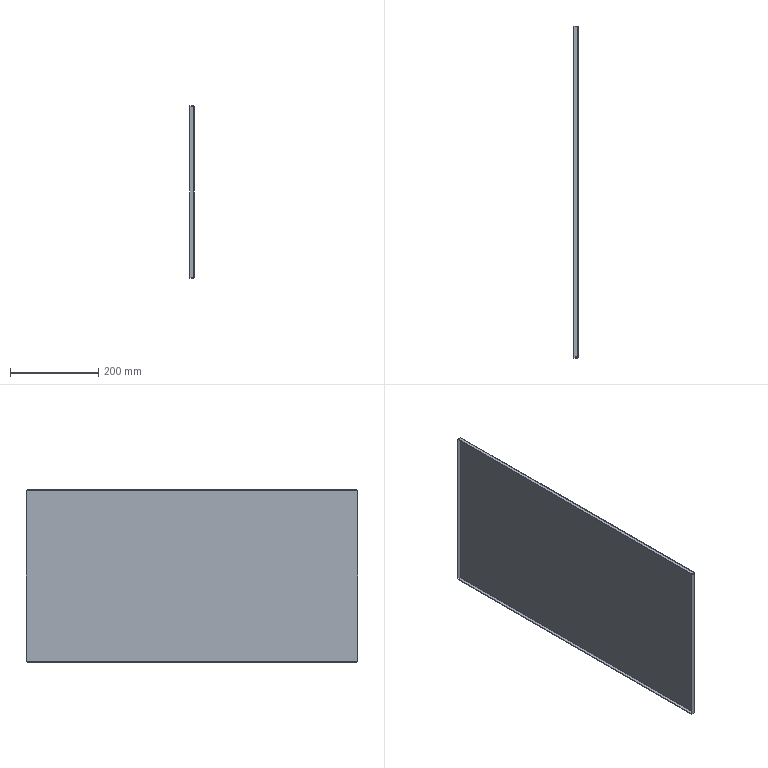Part | SolidWorks | 1 solid | 38 faces | box 10 x 752.001 x 390.001 mm | volume 467554 mm3 | plane 22 | spline 8 | cylinder 8 | commonest cylinder face diameters 0.2 x4 3.2 x4
STEP:
#1=CARTESIAN_POINT('',(-1.5,-374.4,-193.4));
#2=VERTEX_POINT('',#1);
#3=CARTESIAN_POINT('',(-1.5,374.4,-193.4));
#4=VERTEX_POINT('',#3);
#5=CARTESIAN_POINT('',(-1.5,-374.4,-193.4));
#6=DIRECTION('',(0.,1.,0.));
#7=VECTOR('',#6,1000.);
#8=LINE('',#5,#7);
#9=EDGE_CURVE('',#2,#4,#8,.T.);
#10=ORIENTED_EDGE('',*,*,#9,.F.);
#11=CARTESIAN_POINT('',(-1.5,-374.4,193.4));
#12=VERTEX_POINT('',#11);
#13=CARTESIAN_POINT('',(-1.5,-374.4,193.4));
#14=DIRECTION('',(0.,0.,-1.));
#15=VECTOR('',#14,1000.);
#16=LINE('',#13,#15);
#17=EDGE_CURVE('',#12,#2,#16,.T.);
#18=ORIENTED_EDGE('',*,*,#17,.F.);
#19=CARTESIAN_POINT('',(-1.5,374.4,193.4));
#20=VERTEX_POINT('',#19);
#21=CARTESIAN_POINT('',(-1.5,374.4,193.4));
#22=DIRECTION('',(0.,-1.,0.));
#23=VECTOR('',#22,1000.);
#24=LINE('',#21,#23);
#25=EDGE_CURVE('',#20,#12,#24,.T.);
#26=ORIENTED_EDGE('',*,*,#25,.F.);
#27=CARTESIAN_POINT('',(-1.5,374.4,-193.4));
#28=DIRECTION('',(0.,0.,1.));
#29=VECTOR('',#28,1000.);
#30=LINE('',#27,#29);
#31=EDGE_CURVE('',#4,#20,#30,.T.);
#32=ORIENTED_EDGE('',*,*,#31,.F.);
#33=EDGE_LOOP('',(#10,#18,#26,#32));
#34=FACE_OUTER_BOUND('',#33,.T.);
#35=CARTESIAN_POINT('',(-1.5,0.,0.));
#36=DIRECTION('',(1.,0.,0.));
#37=DIRECTION('',(0.,0.,-1.));
#38=AXIS2_PLACEMENT_3D('',#35,#36,#37);
#39=PLANE('',#38);
#40=ADVANCED_FACE('',(#34),#39,.F.);
#41=CARTESIAN_POINT('',(0.,-374.4,193.4));
#42=VERTEX_POINT('',#41);
#43=CARTESIAN_POINT('',(0.,-374.4,-193.4));
#44=VERTEX_POINT('',#43);
#45=CARTESIAN_POINT('',(0.,-374.4,193.4));
#46=DIRECTION('',(0.,0.,-1.));
#47=VECTOR('',#46,1000.);
#48=LINE('',#45,#47);
#49=EDGE_CURVE('',#42,#44,#48,.T.);
#50=ORIENTED_EDGE('',*,*,#49,.T.);
#51=CARTESIAN_POINT('',(0.,374.4,-193.4));
#52=VERTEX_POINT('',#51);
#53=CARTESIAN_POINT('',(0.,-374.4,-193.4));
#54=DIRECTION('',(0.,1.,0.));
#55=VECTOR('',#54,1000.);
#56=LINE('',#53,#55);
#57=EDGE_CURVE('',#44,#52,#56,.T.);
#58=ORIENTED_EDGE('',*,*,#57,.T.);
#59=CARTESIAN_POINT('',(0.,374.4,193.4));
#60=VERTEX_POINT('',#59);
#61=CARTESIAN_POINT('',(0.,374.4,-193.4));
#62=DIRECTION('',(0.,0.,1.));
#63=VECTOR('',#62,1000.);
#64=LINE('',#61,#63);
#65=EDGE_CURVE('',#52,#60,#64,.T.);
#66=ORIENTED_EDGE('',*,*,#65,.T.);
#67=CARTESIAN_POINT('',(0.,374.4,193.4));
#68=DIRECTION('',(0.,-1.,0.));
#69=VECTOR('',#68,1000.);
#70=LINE('',#67,#69);
#71=EDGE_CURVE('',#60,#42,#70,.T.);
#72=ORIENTED_EDGE('',*,*,#71,.T.);
#73=EDGE_LOOP('',(#50,#58,#66,#72));
#74=FACE_OUTER_BOUND('',#73,.T.);
#75=CARTESIAN_POINT('',(0.,0.,0.));
#76=DIRECTION('',(1.,0.,0.));
#77=DIRECTION('',(0.,0.,-1.));
#78=AXIS2_PLACEMENT_3D('',#75,#76,#77);
#79=PLANE('',#78);
#80=ADVANCED_FACE('',(#74),#79,.T.);
#81=CARTESIAN_POINT('',(-1.6,376.,192.793));
#82=VERTEX_POINT('',#81);
#83=CARTESIAN_POINT('',(-1.6,374.5,192.793));
#84=VERTEX_POINT('',#83);
#85=CARTESIAN_POINT('',(-1.6,374.5,192.793));
#86=DIRECTION('',(0.,-1.,0.));
#87=VECTOR('',#86,1000.);
#88=LINE('',#85,#87);
#89=EDGE_CURVE('',#82,#84,#88,.T.);
#90=ORIENTED_EDGE('',*,*,#89,.T.);
#91=CARTESIAN_POINT('',(-1.5,374.4,193.4));
#92=CARTESIAN_POINT('',(-1.5,374.426,193.299));
#93=CARTESIAN_POINT('',(-1.511,374.452,193.198));
#94=CARTESIAN_POINT('',(-1.548,374.489,192.995));
#95=CARTESIAN_POINT('',(-1.574,374.5,192.894));
#96=CARTESIAN_POINT('',(-1.6,374.5,192.793));
#97=B_SPLINE_CURVE_WITH_KNOTS('',3,(#91,#92,#93,#94,#95,#96),.UNSPECIFIED.,.F.,.F.,(4,2,4),(0.,0.5,1.),.UNSPECIFIED.);
#98=EDGE_CURVE('',#20,#84,#97,.T.);
#99=ORIENTED_EDGE('',*,*,#98,.F.);
#100=CARTESIAN_POINT('',(-1.5,374.4,193.4));
#101=DIRECTION('',(1.,0.,0.));
#102=VECTOR('',#101,1000.);
#103=LINE('',#100,#102);
#104=EDGE_CURVE('',#20,#60,#103,.T.);
#105=ORIENTED_EDGE('',*,*,#104,.T.);
#106=CARTESIAN_POINT('',(0.,374.4,193.4));
#107=CARTESIAN_POINT('',(0.,374.612,193.349));
#108=CARTESIAN_POINT('',(-0.04048,374.815,193.3));
#109=CARTESIAN_POINT('',(-0.2012,375.205,193.198));
#110=CARTESIAN_POINT('',(-0.3186,375.381,193.148));
#111=CARTESIAN_POINT('',(-0.5418,375.605,193.071));
#112=CARTESIAN_POINT('',(-0.6225,375.671,193.046));
#113=CARTESIAN_POINT('',(-0.7959,375.787,192.996));
#114=CARTESIAN_POINT('',(-0.8897,375.838,192.97));
#115=CARTESIAN_POINT('',(-1.18,375.958,192.894));
#116=CARTESIAN_POINT('',(-1.388,376.,192.844));
#117=CARTESIAN_POINT('',(-1.6,376.,192.793));
#118=B_SPLINE_CURVE_WITH_KNOTS('',3,(#106,#107,#108,#109,#110,#111,#112,#113,#114,#115,#116,#117),.UNSPECIFIED.,.F.,.F.,(4,2,2,2,2,4),(0.,0.0006399,0.00128,0.0016,0.00192,0.00256),.UNSPECIFIED.);
#119=EDGE_CURVE('',#60,#82,#118,.T.);
#120=ORIENTED_EDGE('',*,*,#119,.T.);
#121=EDGE_LOOP('',(#90,#99,#105,#120));
#122=FACE_OUTER_BOUND('',#121,.T.);
#123=CARTESIAN_POINT('',(0.015,374.4,193.4));
#124=CARTESIAN_POINT('',(0.015,374.611,193.349));
#125=CARTESIAN_POINT('',(-0.02703,374.823,193.299));
#126=CARTESIAN_POINT('',(-0.1888,375.213,193.198));
#127=CARTESIAN_POINT('',(-0.3085,375.392,193.147));
#128=CARTESIAN_POINT('',(-0.6075,375.691,193.046));
#129=CARTESIAN_POINT('',(-0.7867,375.811,192.995));
#130=CARTESIAN_POINT('',(-1.177,375.973,192.894));
#131=CARTESIAN_POINT('',(-1.389,376.015,192.843));
#132=CARTESIAN_POINT('',(-1.6,376.015,192.793));
#133=CARTESIAN_POINT('',(0.,374.4,193.4));
#134=CARTESIAN_POINT('',(0.,374.609,193.349));
#135=CARTESIAN_POINT('',(-0.04164,374.819,193.299));
#136=CARTESIAN_POINT('',(-0.2019,375.206,193.198));
#137=CARTESIAN_POINT('',(-0.3205,375.383,193.147));
#138=CARTESIAN_POINT('',(-0.6167,375.679,193.046));
#139=CARTESIAN_POINT('',(-0.7942,375.798,192.995));
#140=CARTESIAN_POINT('',(-1.181,375.958,192.894));
#141=CARTESIAN_POINT('',(-1.391,376.,192.843));
#142=CARTESIAN_POINT('',(-1.6,376.,192.793));
#143=CARTESIAN_POINT('',(-1.5,374.4,193.4));
#144=CARTESIAN_POINT('',(-1.5,374.413,193.349));
#145=CARTESIAN_POINT('',(-1.503,374.426,193.299));
#146=CARTESIAN_POINT('',(-1.513,374.45,193.198));
#147=CARTESIAN_POINT('',(-1.52,374.461,193.147));
#148=CARTESIAN_POINT('',(-1.539,374.48,193.046));
#149=CARTESIAN_POINT('',(-1.55,374.487,192.995));
#150=CARTESIAN_POINT('',(-1.574,374.497,192.894));
#151=CARTESIAN_POINT('',(-1.587,374.5,192.843));
#152=CARTESIAN_POINT('',(-1.6,374.5,192.793));
#153=B_SPLINE_SURFACE_WITH_KNOTS('',1,3,((#123,#124,#125,#126,#127,#128,#129,#130,#131,#132),(#133,#134,#135,#136,#137,#138,#139,#140,#141,#142),(#143,#144,#145,#146,#147,#148,#149,#150,#151,#152)),.UNSPECIFIED.,.F.,.F.,.F.,(2,1,2),(4,2,2,2,4),(-0.01,0.,1.),(0.,0.25,0.5,0.75,1.),.UNSPECIFIED.);
#154=ADVANCED_FACE('',(#122),#153,.F.);
#155=CARTESIAN_POINT('',(-1.6,374.5,-192.793));
#156=VERTEX_POINT('',#155);
#157=CARTESIAN_POINT('',(-1.6,374.5,-192.793));
#158=CARTESIAN_POINT('',(-1.574,374.5,-192.894));
#159=CARTESIAN_POINT('',(-1.548,374.489,-192.995));
#160=CARTESIAN_POINT('',(-1.511,374.452,-193.198));
#161=CARTESIAN_POINT('',(-1.5,374.426,-193.299));
#162=CARTESIAN_POINT('',(-1.5,374.4,-193.4));
#163=B_SPLINE_CURVE_WITH_KNOTS('',3,(#157,#158,#159,#160,#161,#162),.UNSPECIFIED.,.F.,.F.,(4,2,4),(0.,0.5,1.),.UNSPECIFIED.);
#164=EDGE_CURVE('',#156,#4,#163,.T.);
#165=ORIENTED_EDGE('',*,*,#164,.F.);
#166=CARTESIAN_POINT('',(-1.6,376.,-192.793));
#167=VERTEX_POINT('',#166);
#168=CARTESIAN_POINT('',(-1.6,374.5,-192.793));
#169=DIRECTION('',(0.,-1.,0.));
#170=VECTOR('',#169,1000.);
#171=LINE('',#168,#170);
#172=EDGE_CURVE('',#167,#156,#171,.T.);
#173=ORIENTED_EDGE('',*,*,#172,.F.);
#174=CARTESIAN_POINT('',(-1.6,376.,-192.793));
#175=CARTESIAN_POINT('',(-1.388,376.,-192.844));
#176=CARTESIAN_POINT('',(-1.185,375.96,-192.893));
#177=CARTESIAN_POINT('',(-0.7952,375.799,-192.995));
#178=CARTESIAN_POINT('',(-0.619,375.681,-193.045));
#179=CARTESIAN_POINT('',(-0.3953,375.458,-193.121));
#180=CARTESIAN_POINT('',(-0.329,375.378,-193.147));
#181=CARTESIAN_POINT('',(-0.2128,375.204,-193.197));
#182=CARTESIAN_POINT('',(-0.1625,375.11,-193.223));
#183=CARTESIAN_POINT('',(-0.04195,374.82,-193.299));
#184=CARTESIAN_POINT('',(0.,374.612,-193.349));
#185=CARTESIAN_POINT('',(0.,374.4,-193.4));
#186=B_SPLINE_CURVE_WITH_KNOTS('',3,(#174,#175,#176,#177,#178,#179,#180,#181,#182,#183,#184,#185),.UNSPECIFIED.,.F.,.F.,(4,2,2,2,2,4),(0.,0.0006399,0.00128,0.0016,0.00192,0.00256),.UNSPECIFIED.);
#187=EDGE_CURVE('',#167,#52,#186,.T.);
#188=ORIENTED_EDGE('',*,*,#187,.T.);
#189=CARTESIAN_POINT('',(-1.5,374.4,-193.4));
#190=DIRECTION('',(1.,0.,0.));
#191=VECTOR('',#190,1000.);
#192=LINE('',#189,#191);
#193=EDGE_CURVE('',#4,#52,#192,.T.);
#194=ORIENTED_EDGE('',*,*,#193,.F.);
#195=EDGE_LOOP('',(#165,#173,#188,#194));
#196=FACE_OUTER_BOUND('',#195,.T.);
#197=CARTESIAN_POINT('',(-1.6,376.015,-192.793));
#198=CARTESIAN_POINT('',(-1.389,376.015,-192.843));
#199=CARTESIAN_POINT('',(-1.177,375.973,-192.894));
#200=CARTESIAN_POINT('',(-0.7867,375.811,-192.995));
#201=CARTESIAN_POINT('',(-0.6075,375.691,-193.046));
#202=CARTESIAN_POINT('',(-0.3085,375.392,-193.147));
#203=CARTESIAN_POINT('',(-0.1888,375.213,-193.198));
#204=CARTESIAN_POINT('',(-0.02703,374.823,-193.299));
#205=CARTESIAN_POINT('',(0.015,374.611,-193.349));
#206=CARTESIAN_POINT('',(0.015,374.4,-193.4));
#207=CARTESIAN_POINT('',(-1.6,376.,-192.793));
#208=CARTESIAN_POINT('',(-1.391,376.,-192.843));
#209=CARTESIAN_POINT('',(-1.181,375.958,-192.894));
#210=CARTESIAN_POINT('',(-0.7942,375.798,-192.995));
#211=CARTESIAN_POINT('',(-0.6167,375.679,-193.046));
#212=CARTESIAN_POINT('',(-0.3205,375.383,-193.147));
#213=CARTESIAN_POINT('',(-0.2019,375.206,-193.198));
#214=CARTESIAN_POINT('',(-0.04164,374.819,-193.299));
#215=CARTESIAN_POINT('',(0.,374.609,-193.349));
#216=CARTESIAN_POINT('',(0.,374.4,-193.4));
#217=CARTESIAN_POINT('',(-1.6,374.5,-192.793));
#218=CARTESIAN_POINT('',(-1.587,374.5,-192.843));
#219=CARTESIAN_POINT('',(-1.574,374.497,-192.894));
#220=CARTESIAN_POINT('',(-1.55,374.487,-192.995));
#221=CARTESIAN_POINT('',(-1.539,374.48,-193.046));
#222=CARTESIAN_POINT('',(-1.52,374.461,-193.147));
#223=CARTESIAN_POINT('',(-1.513,374.45,-193.198));
#224=CARTESIAN_POINT('',(-1.503,374.426,-193.299));
#225=CARTESIAN_POINT('',(-1.5,374.413,-193.349));
#226=CARTESIAN_POINT('',(-1.5,374.4,-193.4));
#227=B_SPLINE_SURFACE_WITH_KNOTS('',1,3,((#197,#198,#199,#200,#201,#202,#203,#204,#205,#206),(#207,#208,#209,#210,#211,#212,#213,#214,#215,#216),(#217,#218,#219,#220,#221,#222,#223,#224,#225,#226)),.UNSPECIFIED.,.F.,.F.,.F.,(2,1,2),(4,2,2,2,4),(-0.01,0.,1.),(0.,0.25,0.5,0.75,1.),.UNSPECIFIED.);
#228=ADVANCED_FACE('',(#196),#227,.F.);
#229=ORIENTED_EDGE('',*,*,#65,.F.);
#230=ORIENTED_EDGE('',*,*,#187,.F.);
#231=CARTESIAN_POINT('',(-1.6,376.,0.));
#232=DIRECTION('',(0.,0.,-1.));
#233=VECTOR('',#232,1000.);
#234=LINE('',#231,#233);
#235=EDGE_CURVE('',#82,#167,#234,.T.);
#236=ORIENTED_EDGE('',*,*,#235,.F.);
#237=ORIENTED_EDGE('',*,*,#119,.F.);
#238=EDGE_LOOP('',(#229,#230,#236,#237));
#239=FACE_OUTER_BOUND('',#238,.T.);
#240=CARTESIAN_POINT('',(-1.6,374.4,-193.4));
#241=DIRECTION('',(0.,0.,-1.));
#242=DIRECTION('',(0.,1.,0.));
#243=AXIS2_PLACEMENT_3D('',#240,#241,#242);
#244=CYLINDRICAL_SURFACE('',#243,1.6);
#245=ADVANCED_FACE('',(#239),#244,.T.);
#246=ORIENTED_EDGE('',*,*,#31,.T.);
#247=ORIENTED_EDGE('',*,*,#98,.T.);
#248=CARTESIAN_POINT('',(-1.6,374.5,195.));
#249=DIRECTION('',(0.,0.,-1.));
#250=VECTOR('',#249,1000.);
#251=LINE('',#248,#250);
#252=EDGE_CURVE('',#84,#156,#251,.T.);
#253=ORIENTED_EDGE('',*,*,#252,.T.);
#254=ORIENTED_EDGE('',*,*,#164,.T.);
#255=EDGE_LOOP('',(#246,#247,#253,#254));
#256=FACE_OUTER_BOUND('',#255,.T.);
#257=CARTESIAN_POINT('',(-1.6,374.4,-193.4));
#258=DIRECTION('',(0.,0.,-1.));
#259=DIRECTION('',(0.,1.,0.));
#260=AXIS2_PLACEMENT_3D('',#257,#258,#259);
#261=CYLINDRICAL_SURFACE('',#260,0.1);
#262=ADVANCED_FACE('',(#256),#261,.F.);
#263=CARTESIAN_POINT('',(-10.,374.5,192.793));
#264=VERTEX_POINT('',#263);
#265=CARTESIAN_POINT('',(-10.,376.,192.793));
#266=VERTEX_POINT('',#265);
#267=CARTESIAN_POINT('',(-10.,376.,192.793));
#268=DIRECTION('',(0.,1.,0.));
#269=VECTOR('',#268,1000.);
#270=LINE('',#267,#269);
#271=EDGE_CURVE('',#264,#266,#270,.T.);
#272=ORIENTED_EDGE('',*,*,#271,.F.);
#273=CARTESIAN_POINT('',(0.,374.5,192.793));
#274=DIRECTION('',(-1.,0.,0.));
#275=VECTOR('',#274,1000.);
#276=LINE('',#273,#275);
#277=EDGE_CURVE('',#84,#264,#276,.T.);
#278=ORIENTED_EDGE('',*,*,#277,.F.);
#279=ORIENTED_EDGE('',*,*,#89,.F.);
#280=CARTESIAN_POINT('',(0.,376.,192.793));
#281=DIRECTION('',(1.,0.,0.));
#282=VECTOR('',#281,1000.);
#283=LINE('',#280,#282);
#284=EDGE_CURVE('',#266,#82,#283,.T.);
#285=ORIENTED_EDGE('',*,*,#284,.F.);
#286=EDGE_LOOP('',(#272,#278,#279,#285));
#287=FACE_OUTER_BOUND('',#286,.T.);
#288=CARTESIAN_POINT('',(-1.5,374.5,192.793));
#289=DIRECTION('',(0.,0.,1.));
#290=DIRECTION('',(1.,0.,0.));
#291=AXIS2_PLACEMENT_3D('',#288,#289,#290);
#292=PLANE('',#291);
#293=ADVANCED_FACE('',(#287),#292,.T.);
#294=CARTESIAN_POINT('',(-10.,376.,-192.793));
#295=VERTEX_POINT('',#294);
#296=CARTESIAN_POINT('',(-1.5,376.,-192.793));
#297=DIRECTION('',(1.,0.,0.));
#298=VECTOR('',#297,1000.);
#299=LINE('',#296,#298);
#300=EDGE_CURVE('',#295,#167,#299,.T.);
#301=ORIENTED_EDGE('',*,*,#300,.F.);
#302=CARTESIAN_POINT('',(-10.,376.,-195.));
#303=DIRECTION('',(0.,0.,-1.));
#304=VECTOR('',#303,1000.);
#305=LINE('',#302,#304);
#306=EDGE_CURVE('',#266,#295,#305,.T.);
#307=ORIENTED_EDGE('',*,*,#306,.F.);
#308=ORIENTED_EDGE('',*,*,#284,.T.);
#309=ORIENTED_EDGE('',*,*,#235,.T.);
#310=EDGE_LOOP('',(#301,#307,#308,#309));
#311=FACE_OUTER_BOUND('',#310,.T.);
#312=CARTESIAN_POINT('',(0.,376.,0.));
#313=DIRECTION('',(0.,1.,0.));
#314=DIRECTION('',(-1.,0.,0.));
#315=AXIS2_PLACEMENT_3D('',#312,#313,#314);
#316=PLANE('',#315);
#317=ADVANCED_FACE('',(#311),#316,.T.);
#318=CARTESIAN_POINT('',(-10.,374.5,-192.793));
#319=VERTEX_POINT('',#318);
#320=CARTESIAN_POINT('',(-10.,374.5,0.));
#321=DIRECTION('',(0.,0.,-1.));
#322=VECTOR('',#321,1000.);
#323=LINE('',#320,#322);
#324=EDGE_CURVE('',#264,#319,#323,.T.);
#325=ORIENTED_EDGE('',*,*,#324,.T.);
#326=CARTESIAN_POINT('',(-1.5,374.5,-192.793));
#327=DIRECTION('',(-1.,0.,0.));
#328=VECTOR('',#327,1000.);
#329=LINE('',#326,#328);
#330=EDGE_CURVE('',#156,#319,#329,.T.);
#331=ORIENTED_EDGE('',*,*,#330,.F.);
#332=ORIENTED_EDGE('',*,*,#252,.F.);
#333=ORIENTED_EDGE('',*,*,#277,.T.);
#334=EDGE_LOOP('',(#325,#331,#332,#333));
#335=FACE_OUTER_BOUND('',#334,.T.);
#336=CARTESIAN_POINT('',(0.,374.5,0.));
#337=DIRECTION('',(0.,1.,0.));
#338=DIRECTION('',(-1.,0.,0.));
#339=AXIS2_PLACEMENT_3D('',#336,#337,#338);
#340=PLANE('',#339);
#341=ADVANCED_FACE('',(#335),#340,.F.);
#342=CARTESIAN_POINT('',(-10.,374.5,-192.793));
#343=DIRECTION('',(0.,1.,0.));
#344=VECTOR('',#343,1000.);
#345=LINE('',#342,#344);
#346=EDGE_CURVE('',#319,#295,#345,.T.);
#347=ORIENTED_EDGE('',*,*,#346,.F.);
#348=ORIENTED_EDGE('',*,*,#324,.F.);
#349=ORIENTED_EDGE('',*,*,#271,.T.);
#350=ORIENTED_EDGE('',*,*,#306,.T.);
#351=EDGE_LOOP('',(#347,#348,#349,#350));
#352=FACE_OUTER_BOUND('',#351,.T.);
#353=CARTESIAN_POINT('',(-10.,376.,-195.));
#354=DIRECTION('',(-1.,0.,0.));
#355=DIRECTION('',(0.,-1.,0.));
#356=AXIS2_PLACEMENT_3D('',#353,#354,#355);
#357=PLANE('',#356);
#358=ADVANCED_FACE('',(#352),#357,.T.);
#359=ORIENTED_EDGE('',*,*,#330,.T.);
#360=ORIENTED_EDGE('',*,*,#346,.T.);
#361=ORIENTED_EDGE('',*,*,#300,.T.);
#362=ORIENTED_EDGE('',*,*,#172,.T.);
#363=EDGE_LOOP('',(#359,#360,#361,#362));
#364=FACE_OUTER_BOUND('',#363,.T.);
#365=CARTESIAN_POINT('',(-1.5,374.5,-192.793));
#366=DIRECTION('',(0.,0.,1.));
#367=DIRECTION('',(1.,0.,0.));
#368=AXIS2_PLACEMENT_3D('',#365,#366,#367);
#369=PLANE('',#368);
#370=ADVANCED_FACE('',(#364),#369,.F.);
#371=CARTESIAN_POINT('',(-1.6,-373.793,195.));
#372=VERTEX_POINT('',#371);
#373=CARTESIAN_POINT('',(-1.6,-373.793,193.5));
#374=VERTEX_POINT('',#373);
#375=CARTESIAN_POINT('',(-1.6,-373.793,193.5));
#376=DIRECTION('',(0.,0.,-1.));
#377=VECTOR('',#376,1000.);
#378=LINE('',#375,#377);
#379=EDGE_CURVE('',#372,#374,#378,.T.);
#380=ORIENTED_EDGE('',*,*,#379,.T.);
#381=CARTESIAN_POINT('',(-1.5,-374.4,193.4));
#382=CARTESIAN_POINT('',(-1.5,-374.299,193.426));
#383=CARTESIAN_POINT('',(-1.511,-374.198,193.452));
#384=CARTESIAN_POINT('',(-1.548,-373.995,193.489));
#385=CARTESIAN_POINT('',(-1.574,-373.894,193.5));
#386=CARTESIAN_POINT('',(-1.6,-373.793,193.5));
#387=B_SPLINE_CURVE_WITH_KNOTS('',3,(#381,#382,#383,#384,#385,#386),.UNSPECIFIED.,.F.,.F.,(4,2,4),(0.,0.5,1.),.UNSPECIFIED.);
#388=EDGE_CURVE('',#12,#374,#387,.T.);
#389=ORIENTED_EDGE('',*,*,#388,.F.);
#390=CARTESIAN_POINT('',(-1.5,-374.4,193.4));
#391=DIRECTION('',(1.,0.,0.));
#392=VECTOR('',#391,1000.);
#393=LINE('',#390,#392);
#394=EDGE_CURVE('',#12,#42,#393,.T.);
#395=ORIENTED_EDGE('',*,*,#394,.T.);
#396=CARTESIAN_POINT('',(0.,-374.4,193.4));
#397=CARTESIAN_POINT('',(0.,-374.349,193.612));
#398=CARTESIAN_POINT('',(-0.04048,-374.3,193.815));
#399=CARTESIAN_POINT('',(-0.2012,-374.198,194.205));
#400=CARTESIAN_POINT('',(-0.3186,-374.148,194.381));
#401=CARTESIAN_POINT('',(-0.5418,-374.071,194.605));
#402=CARTESIAN_POINT('',(-0.6225,-374.046,194.671));
#403=CARTESIAN_POINT('',(-0.7959,-373.996,194.787));
#404=CARTESIAN_POINT('',(-0.8897,-373.97,194.838));
#405=CARTESIAN_POINT('',(-1.18,-373.894,194.958));
#406=CARTESIAN_POINT('',(-1.388,-373.844,195.));
#407=CARTESIAN_POINT('',(-1.6,-373.793,195.));
#408=B_SPLINE_CURVE_WITH_KNOTS('',3,(#396,#397,#398,#399,#400,#401,#402,#403,#404,#405,#406,#407),.UNSPECIFIED.,.F.,.F.,(4,2,2,2,2,4),(0.,0.0006399,0.00128,0.0016,0.00192,0.00256),.UNSPECIFIED.);
#409=EDGE_CURVE('',#42,#372,#408,.T.);
#410=ORIENTED_EDGE('',*,*,#409,.T.);
#411=EDGE_LOOP('',(#380,#389,#395,#410));
#412=FACE_OUTER_BOUND('',#411,.T.);
#413=CARTESIAN_POINT('',(0.015,-374.4,193.4));
#414=CARTESIAN_POINT('',(0.015,-374.349,193.611));
#415=CARTESIAN_POINT('',(-0.02703,-374.299,193.823));
#416=CARTESIAN_POINT('',(-0.1888,-374.198,194.213));
#417=CARTESIAN_POINT('',(-0.3085,-374.147,194.392));
#418=CARTESIAN_POINT('',(-0.6075,-374.046,194.691));
#419=CARTESIAN_POINT('',(-0.7867,-373.995,194.811));
#420=CARTESIAN_POINT('',(-1.177,-373.894,194.973));
#421=CARTESIAN_POINT('',(-1.389,-373.843,195.015));
#422=CARTESIAN_POINT('',(-1.6,-373.793,195.015));
#423=CARTESIAN_POINT('',(0.,-374.4,193.4));
#424=CARTESIAN_POINT('',(0.,-374.349,193.609));
#425=CARTESIAN_POINT('',(-0.04164,-374.299,193.819));
#426=CARTESIAN_POINT('',(-0.2019,-374.198,194.206));
#427=CARTESIAN_POINT('',(-0.3205,-374.147,194.383));
#428=CARTESIAN_POINT('',(-0.6167,-374.046,194.679));
#429=CARTESIAN_POINT('',(-0.7942,-373.995,194.798));
#430=CARTESIAN_POINT('',(-1.181,-373.894,194.958));
#431=CARTESIAN_POINT('',(-1.391,-373.843,195.));
#432=CARTESIAN_POINT('',(-1.6,-373.793,195.));
#433=CARTESIAN_POINT('',(-1.5,-374.4,193.4));
#434=CARTESIAN_POINT('',(-1.5,-374.349,193.413));
#435=CARTESIAN_POINT('',(-1.503,-374.299,193.426));
#436=CARTESIAN_POINT('',(-1.513,-374.198,193.45));
#437=CARTESIAN_POINT('',(-1.52,-374.147,193.461));
#438=CARTESIAN_POINT('',(-1.539,-374.046,193.48));
#439=CARTESIAN_POINT('',(-1.55,-373.995,193.487));
#440=CARTESIAN_POINT('',(-1.574,-373.894,193.497));
#441=CARTESIAN_POINT('',(-1.587,-373.843,193.5));
#442=CARTESIAN_POINT('',(-1.6,-373.793,193.5));
#443=B_SPLINE_SURFACE_WITH_KNOTS('',1,3,((#413,#414,#415,#416,#417,#418,#419,#420,#421,#422),(#423,#424,#425,#426,#427,#428,#429,#430,#431,#432),(#433,#434,#435,#436,#437,#438,#439,#440,#441,#442)),.UNSPECIFIED.,.F.,.F.,.F.,(2,1,2),(4,2,2,2,4),(-0.01,0.,1.),(0.,0.25,0.5,0.75,1.),.UNSPECIFIED.);
#444=ADVANCED_FACE('',(#412),#443,.F.);
#445=CARTESIAN_POINT('',(-1.6,373.793,193.5));
#446=VERTEX_POINT('',#445);
#447=CARTESIAN_POINT('',(-1.6,373.793,193.5));
#448=CARTESIAN_POINT('',(-1.574,373.894,193.5));
#449=CARTESIAN_POINT('',(-1.548,373.995,193.489));
#450=CARTESIAN_POINT('',(-1.511,374.198,193.452));
#451=CARTESIAN_POINT('',(-1.5,374.299,193.426));
#452=CARTESIAN_POINT('',(-1.5,374.4,193.4));
#453=B_SPLINE_CURVE_WITH_KNOTS('',3,(#447,#448,#449,#450,#451,#452),.UNSPECIFIED.,.F.,.F.,(4,2,4),(0.,0.5,1.),.UNSPECIFIED.);
#454=EDGE_CURVE('',#446,#20,#453,.T.);
#455=ORIENTED_EDGE('',*,*,#454,.F.);
#456=CARTESIAN_POINT('',(-1.6,373.793,195.));
#457=VERTEX_POINT('',#456);
#458=CARTESIAN_POINT('',(-1.6,373.793,193.5));
#459=DIRECTION('',(0.,0.,-1.));
#460=VECTOR('',#459,1000.);
#461=LINE('',#458,#460);
#462=EDGE_CURVE('',#457,#446,#461,.T.);
#463=ORIENTED_EDGE('',*,*,#462,.F.);
#464=CARTESIAN_POINT('',(-1.6,373.793,195.));
#465=CARTESIAN_POINT('',(-1.388,373.844,195.));
#466=CARTESIAN_POINT('',(-1.185,373.893,194.96));
#467=CARTESIAN_POINT('',(-0.7952,373.995,194.799));
#468=CARTESIAN_POINT('',(-0.619,374.045,194.681));
#469=CARTESIAN_POINT('',(-0.3953,374.121,194.458));
#470=CARTESIAN_POINT('',(-0.329,374.147,194.378));
#471=CARTESIAN_POINT('',(-0.2128,374.197,194.204));
#472=CARTESIAN_POINT('',(-0.1625,374.223,194.11));
#473=CARTESIAN_POINT('',(-0.04195,374.299,193.82));
#474=CARTESIAN_POINT('',(0.,374.349,193.612));
#475=CARTESIAN_POINT('',(0.,374.4,193.4));
#476=B_SPLINE_CURVE_WITH_KNOTS('',3,(#464,#465,#466,#467,#468,#469,#470,#471,#472,#473,#474,#475),.UNSPECIFIED.,.F.,.F.,(4,2,2,2,2,4),(0.,0.0006399,0.00128,0.0016,0.00192,0.00256),.UNSPECIFIED.);
#477=EDGE_CURVE('',#457,#60,#476,.T.);
#478=ORIENTED_EDGE('',*,*,#477,.T.);
#479=ORIENTED_EDGE('',*,*,#104,.F.);
#480=EDGE_LOOP('',(#455,#463,#478,#479));
#481=FACE_OUTER_BOUND('',#480,.T.);
#482=CARTESIAN_POINT('',(-1.6,373.793,195.015));
#483=CARTESIAN_POINT('',(-1.389,373.843,195.015));
#484=CARTESIAN_POINT('',(-1.177,373.894,194.973));
#485=CARTESIAN_POINT('',(-0.7867,373.995,194.811));
#486=CARTESIAN_POINT('',(-0.6075,374.046,194.691));
#487=CARTESIAN_POINT('',(-0.3085,374.147,194.392));
#488=CARTESIAN_POINT('',(-0.1888,374.198,194.213));
#489=CARTESIAN_POINT('',(-0.02703,374.299,193.823));
#490=CARTESIAN_POINT('',(0.015,374.349,193.611));
#491=CARTESIAN_POINT('',(0.015,374.4,193.4));
#492=CARTESIAN_POINT('',(-1.6,373.793,195.));
#493=CARTESIAN_POINT('',(-1.391,373.843,195.));
#494=CARTESIAN_POINT('',(-1.181,373.894,194.958));
#495=CARTESIAN_POINT('',(-0.7942,373.995,194.798));
#496=CARTESIAN_POINT('',(-0.6167,374.046,194.679));
#497=CARTESIAN_POINT('',(-0.3205,374.147,194.383));
#498=CARTESIAN_POINT('',(-0.2019,374.198,194.206));
#499=CARTESIAN_POINT('',(-0.04164,374.299,193.819));
#500=CARTESIAN_POINT('',(0.,374.349,193.609));
#501=CARTESIAN_POINT('',(0.,374.4,193.4));
#502=CARTESIAN_POINT('',(-1.6,373.793,193.5));
#503=CARTESIAN_POINT('',(-1.587,373.843,193.5));
#504=CARTESIAN_POINT('',(-1.574,373.894,193.497));
#505=CARTESIAN_POINT('',(-1.55,373.995,193.487));
#506=CARTESIAN_POINT('',(-1.539,374.046,193.48));
#507=CARTESIAN_POINT('',(-1.52,374.147,193.461));
#508=CARTESIAN_POINT('',(-1.513,374.198,193.45));
#509=CARTESIAN_POINT('',(-1.503,374.299,193.426));
#510=CARTESIAN_POINT('',(-1.5,374.349,193.413));
#511=CARTESIAN_POINT('',(-1.5,374.4,193.4));
#512=B_SPLINE_SURFACE_WITH_KNOTS('',1,3,((#482,#483,#484,#485,#486,#487,#488,#489,#490,#491),(#492,#493,#494,#495,#496,#497,#498,#499,#500,#501),(#502,#503,#504,#505,#506,#507,#508,#509,#510,#511)),.UNSPECIFIED.,.F.,.F.,.F.,(2,1,2),(4,2,2,2,4),(-0.01,0.,1.),(0.,0.25,0.5,0.75,1.),.UNSPECIFIED.);
#513=ADVANCED_FACE('',(#481),#512,.F.);
#514=ORIENTED_EDGE('',*,*,#71,.F.);
#515=ORIENTED_EDGE('',*,*,#477,.F.);
#516=CARTESIAN_POINT('',(-1.6,-376.,195.));
#517=DIRECTION('',(0.,-1.,0.));
#518=VECTOR('',#517,1000.);
#519=LINE('',#516,#518);
#520=EDGE_CURVE('',#457,#372,#519,.T.);
#521=ORIENTED_EDGE('',*,*,#520,.T.);
#522=ORIENTED_EDGE('',*,*,#409,.F.);
#523=EDGE_LOOP('',(#514,#515,#521,#522));
#524=FACE_OUTER_BOUND('',#523,.T.);
#525=CARTESIAN_POINT('',(-1.6,374.4,193.4));
#526=DIRECTION('',(0.,1.,0.));
#527=DIRECTION('',(0.,0.,1.));
#528=AXIS2_PLACEMENT_3D('',#525,#526,#527);
#529=CYLINDRICAL_SURFACE('',#528,1.6);
#530=ADVANCED_FACE('',(#524),#529,.T.);
#531=ORIENTED_EDGE('',*,*,#25,.T.);
#532=ORIENTED_EDGE('',*,*,#388,.T.);
#533=CARTESIAN_POINT('',(-1.6,-376.,193.5));
#534=DIRECTION('',(0.,1.,0.));
#535=VECTOR('',#534,1000.);
#536=LINE('',#533,#535);
#537=EDGE_CURVE('',#374,#446,#536,.T.);
#538=ORIENTED_EDGE('',*,*,#537,.T.);
#539=ORIENTED_EDGE('',*,*,#454,.T.);
#540=EDGE_LOOP('',(#531,#532,#538,#539));
#541=FACE_OUTER_BOUND('',#540,.T.);
#542=CARTESIAN_POINT('',(-1.6,374.4,193.4));
#543=DIRECTION('',(0.,1.,0.));
#544=DIRECTION('',(0.,0.,1.));
#545=AXIS2_PLACEMENT_3D('',#542,#543,#544);
#546=CYLINDRICAL_SURFACE('',#545,0.1);
#547=ADVANCED_FACE('',(#541),#546,.F.);
#548=CARTESIAN_POINT('',(-10.,-373.793,193.5));
#549=VERTEX_POINT('',#548);
#550=CARTESIAN_POINT('',(-10.,-373.793,195.));
#551=VERTEX_POINT('',#550);
#552=CARTESIAN_POINT('',(-10.,-373.793,195.));
#553=DIRECTION('',(0.,0.,1.));
#554=VECTOR('',#553,1000.);
#555=LINE('',#552,#554);
#556=EDGE_CURVE('',#549,#551,#555,.T.);
#557=ORIENTED_EDGE('',*,*,#556,.F.);
#558=CARTESIAN_POINT('',(0.,-373.793,193.5));
#559=DIRECTION('',(-1.,0.,0.));
#560=VECTOR('',#559,1000.);
#561=LINE('',#558,#560);
#562=EDGE_CURVE('',#374,#549,#561,.T.);
#563=ORIENTED_EDGE('',*,*,#562,.F.);
#564=ORIENTED_EDGE('',*,*,#379,.F.);
#565=CARTESIAN_POINT('',(-1.5,-373.793,195.));
#566=DIRECTION('',(-1.,0.,0.));
#567=VECTOR('',#566,1000.);
#568=LINE('',#565,#567);
#569=EDGE_CURVE('',#372,#551,#568,.T.);
#570=ORIENTED_EDGE('',*,*,#569,.T.);
#571=EDGE_LOOP('',(#557,#563,#564,#570));
#572=FACE_OUTER_BOUND('',#571,.T.);
#573=CARTESIAN_POINT('',(-1.5,-373.793,193.5));
#574=DIRECTION('',(0.,-1.,0.));
#575=DIRECTION('',(1.,0.,0.));
#576=AXIS2_PLACEMENT_3D('',#573,#574,#575);
#577=PLANE('',#576);
#578=ADVANCED_FACE('',(#572),#577,.T.);
#579=ORIENTED_EDGE('',*,*,#520,.F.);
#580=CARTESIAN_POINT('',(-10.,373.793,195.));
#581=VERTEX_POINT('',#580);
#582=CARTESIAN_POINT('',(0.,373.793,195.));
#583=DIRECTION('',(-1.,0.,0.));
#584=VECTOR('',#583,1000.);
#585=LINE('',#582,#584);
#586=EDGE_CURVE('',#457,#581,#585,.T.);
#587=ORIENTED_EDGE('',*,*,#586,.T.);
#588=CARTESIAN_POINT('',(-10.,-376.,195.));
#589=DIRECTION('',(0.,1.,0.));
#590=VECTOR('',#589,1000.);
#591=LINE('',#588,#590);
#592=EDGE_CURVE('',#551,#581,#591,.T.);
#593=ORIENTED_EDGE('',*,*,#592,.F.);
#594=ORIENTED_EDGE('',*,*,#569,.F.);
#595=EDGE_LOOP('',(#579,#587,#593,#594));
#596=FACE_OUTER_BOUND('',#595,.T.);
#597=CARTESIAN_POINT('',(0.,0.,195.));
#598=DIRECTION('',(0.,0.,-1.));
#599=DIRECTION('',(-1.,0.,0.));
#600=AXIS2_PLACEMENT_3D('',#597,#598,#599);
#601=PLANE('',#600);
#602=ADVANCED_FACE('',(#596),#601,.F.);
#603=CARTESIAN_POINT('',(-10.,373.793,193.5));
#604=VERTEX_POINT('',#603);
#605=CARTESIAN_POINT('',(-1.5,373.793,193.5));
#606=DIRECTION('',(-1.,0.,0.));
#607=VECTOR('',#606,1000.);
#608=LINE('',#605,#607);
#609=EDGE_CURVE('',#446,#604,#608,.T.);
#610=ORIENTED_EDGE('',*,*,#609,.F.);
#611=ORIENTED_EDGE('',*,*,#537,.F.);
#612=ORIENTED_EDGE('',*,*,#562,.T.);
#613=CARTESIAN_POINT('',(-10.,0.,193.5));
#614=DIRECTION('',(0.,1.,0.));
#615=VECTOR('',#614,1000.);
#616=LINE('',#613,#615);
#617=EDGE_CURVE('',#549,#604,#616,.T.);
#618=ORIENTED_EDGE('',*,*,#617,.T.);
#619=EDGE_LOOP('',(#610,#611,#612,#618));
#620=FACE_OUTER_BOUND('',#619,.T.);
#621=CARTESIAN_POINT('',(0.,0.,193.5));
#622=DIRECTION('',(0.,0.,-1.));
#623=DIRECTION('',(-1.,0.,0.));
#624=AXIS2_PLACEMENT_3D('',#621,#622,#623);
#625=PLANE('',#624);
#626=ADVANCED_FACE('',(#620),#625,.T.);
#627=CARTESIAN_POINT('',(-10.,373.793,193.5));
#628=DIRECTION('',(0.,0.,1.));
#629=VECTOR('',#628,1000.);
#630=LINE('',#627,#629);
#631=EDGE_CURVE('',#604,#581,#630,.T.);
#632=ORIENTED_EDGE('',*,*,#631,.F.);
#633=ORIENTED_EDGE('',*,*,#617,.F.);
#634=ORIENTED_EDGE('',*,*,#556,.T.);
#635=ORIENTED_EDGE('',*,*,#592,.T.);
#636=EDGE_LOOP('',(#632,#633,#634,#635));
#637=FACE_OUTER_BOUND('',#636,.T.);
#638=CARTESIAN_POINT('',(-10.,-376.,195.));
#639=DIRECTION('',(-1.,0.,0.));
#640=DIRECTION('',(0.,0.,1.));
#641=AXIS2_PLACEMENT_3D('',#638,#639,#640);
#642=PLANE('',#641);
#643=ADVANCED_FACE('',(#637),#642,.T.);
#644=ORIENTED_EDGE('',*,*,#609,.T.);
#645=ORIENTED_EDGE('',*,*,#631,.T.);
#646=ORIENTED_EDGE('',*,*,#586,.F.);
#647=ORIENTED_EDGE('',*,*,#462,.T.);
#648=EDGE_LOOP('',(#644,#645,#646,#647));
#649=FACE_OUTER_BOUND('',#648,.T.);
#650=CARTESIAN_POINT('',(-1.5,373.793,193.5));
#651=DIRECTION('',(0.,-1.,0.));
#652=DIRECTION('',(1.,0.,0.));
#653=AXIS2_PLACEMENT_3D('',#650,#651,#652);
#654=PLANE('',#653);
#655=ADVANCED_FACE('',(#649),#654,.F.);
#656=CARTESIAN_POINT('',(-1.6,-376.,-192.793));
#657=VERTEX_POINT('',#656);
#658=CARTESIAN_POINT('',(-1.6,-374.5,-192.793));
#659=VERTEX_POINT('',#658);
#660=CARTESIAN_POINT('',(-1.6,-374.5,-192.793));
#661=DIRECTION('',(0.,1.,0.));
#662=VECTOR('',#661,1000.);
#663=LINE('',#660,#662);
#664=EDGE_CURVE('',#657,#659,#663,.T.);
#665=ORIENTED_EDGE('',*,*,#664,.T.);
#666=CARTESIAN_POINT('',(-1.5,-374.4,-193.4));
#667=CARTESIAN_POINT('',(-1.5,-374.426,-193.299));
#668=CARTESIAN_POINT('',(-1.511,-374.452,-193.198));
#669=CARTESIAN_POINT('',(-1.548,-374.489,-192.995));
#670=CARTESIAN_POINT('',(-1.574,-374.5,-192.894));
#671=CARTESIAN_POINT('',(-1.6,-374.5,-192.793));
#672=B_SPLINE_CURVE_WITH_KNOTS('',3,(#666,#667,#668,#669,#670,#671),.UNSPECIFIED.,.F.,.F.,(4,2,4),(0.,0.5,1.),.UNSPECIFIED.);
#673=EDGE_CURVE('',#2,#659,#672,.T.);
#674=ORIENTED_EDGE('',*,*,#673,.F.);
#675=CARTESIAN_POINT('',(-1.5,-374.4,-193.4));
#676=DIRECTION('',(1.,0.,0.));
#677=VECTOR('',#676,1000.);
#678=LINE('',#675,#677);
#679=EDGE_CURVE('',#2,#44,#678,.T.);
#680=ORIENTED_EDGE('',*,*,#679,.T.);
#681=CARTESIAN_POINT('',(0.,-374.4,-193.4));
#682=CARTESIAN_POINT('',(0.,-374.612,-193.349));
#683=CARTESIAN_POINT('',(-0.04048,-374.815,-193.3));
#684=CARTESIAN_POINT('',(-0.2012,-375.205,-193.198));
#685=CARTESIAN_POINT('',(-0.3186,-375.381,-193.148));
#686=CARTESIAN_POINT('',(-0.5418,-375.605,-193.071));
#687=CARTESIAN_POINT('',(-0.6225,-375.671,-193.046));
#688=CARTESIAN_POINT('',(-0.7959,-375.787,-192.996));
#689=CARTESIAN_POINT('',(-0.8897,-375.838,-192.97));
#690=CARTESIAN_POINT('',(-1.18,-375.958,-192.894));
#691=CARTESIAN_POINT('',(-1.388,-376.,-192.844));
#692=CARTESIAN_POINT('',(-1.6,-376.,-192.793));
#693=B_SPLINE_CURVE_WITH_KNOTS('',3,(#681,#682,#683,#684,#685,#686,#687,#688,#689,#690,#691,#692),.UNSPECIFIED.,.F.,.F.,(4,2,2,2,2,4),(0.,0.0006399,0.00128,0.0016,0.00192,0.00256),.UNSPECIFIED.);
#694=EDGE_CURVE('',#44,#657,#693,.T.);
#695=ORIENTED_EDGE('',*,*,#694,.T.);
#696=EDGE_LOOP('',(#665,#674,#680,#695));
#697=FACE_OUTER_BOUND('',#696,.T.);
#698=CARTESIAN_POINT('',(0.015,-374.4,-193.4));
#699=CARTESIAN_POINT('',(0.015,-374.611,-193.349));
#700=CARTESIAN_POINT('',(-0.02703,-374.823,-193.299));
#701=CARTESIAN_POINT('',(-0.1888,-375.213,-193.198));
#702=CARTESIAN_POINT('',(-0.3085,-375.392,-193.147));
#703=CARTESIAN_POINT('',(-0.6075,-375.691,-193.046));
#704=CARTESIAN_POINT('',(-0.7867,-375.811,-192.995));
#705=CARTESIAN_POINT('',(-1.177,-375.973,-192.894));
#706=CARTESIAN_POINT('',(-1.389,-376.015,-192.843));
#707=CARTESIAN_POINT('',(-1.6,-376.015,-192.793));
#708=CARTESIAN_POINT('',(0.,-374.4,-193.4));
#709=CARTESIAN_POINT('',(0.,-374.609,-193.349));
#710=CARTESIAN_POINT('',(-0.04164,-374.819,-193.299));
#711=CARTESIAN_POINT('',(-0.2019,-375.206,-193.198));
#712=CARTESIAN_POINT('',(-0.3205,-375.383,-193.147));
#713=CARTESIAN_POINT('',(-0.6167,-375.679,-193.046));
#714=CARTESIAN_POINT('',(-0.7942,-375.798,-192.995));
#715=CARTESIAN_POINT('',(-1.181,-375.958,-192.894));
#716=CARTESIAN_POINT('',(-1.391,-376.,-192.843));
#717=CARTESIAN_POINT('',(-1.6,-376.,-192.793));
#718=CARTESIAN_POINT('',(-1.5,-374.4,-193.4));
#719=CARTESIAN_POINT('',(-1.5,-374.413,-193.349));
#720=CARTESIAN_POINT('',(-1.503,-374.426,-193.299));
#721=CARTESIAN_POINT('',(-1.513,-374.45,-193.198));
#722=CARTESIAN_POINT('',(-1.52,-374.461,-193.147));
#723=CARTESIAN_POINT('',(-1.539,-374.48,-193.046));
#724=CARTESIAN_POINT('',(-1.55,-374.487,-192.995));
#725=CARTESIAN_POINT('',(-1.574,-374.497,-192.894));
#726=CARTESIAN_POINT('',(-1.587,-374.5,-192.843));
#727=CARTESIAN_POINT('',(-1.6,-374.5,-192.793));
#728=B_SPLINE_SURFACE_WITH_KNOTS('',1,3,((#698,#699,#700,#701,#702,#703,#704,#705,#706,#707),(#708,#709,#710,#711,#712,#713,#714,#715,#716,#717),(#718,#719,#720,#721,#722,#723,#724,#725,#726,#727)),.UNSPECIFIED.,.F.,.F.,.F.,(2,1,2),(4,2,2,2,4),(-0.01,0.,1.),(0.,0.25,0.5,0.75,1.),.UNSPECIFIED.);
#729=ADVANCED_FACE('',(#697),#728,.F.);
#730=CARTESIAN_POINT('',(-1.6,-374.5,192.793));
#731=VERTEX_POINT('',#730);
#732=CARTESIAN_POINT('',(-1.6,-374.5,192.793));
#733=CARTESIAN_POINT('',(-1.574,-374.5,192.894));
#734=CARTESIAN_POINT('',(-1.548,-374.489,192.995));
#735=CARTESIAN_POINT('',(-1.511,-374.452,193.198));
#736=CARTESIAN_POINT('',(-1.5,-374.426,193.299));
#737=CARTESIAN_POINT('',(-1.5,-374.4,193.4));
#738=B_SPLINE_CURVE_WITH_KNOTS('',3,(#732,#733,#734,#735,#736,#737),.UNSPECIFIED.,.F.,.F.,(4,2,4),(0.,0.5,1.),.UNSPECIFIED.);
#739=EDGE_CURVE('',#731,#12,#738,.T.);
#740=ORIENTED_EDGE('',*,*,#739,.F.);
#741=CARTESIAN_POINT('',(-1.6,-376.,192.793));
#742=VERTEX_POINT('',#741);
#743=CARTESIAN_POINT('',(-1.6,-374.5,192.793));
#744=DIRECTION('',(0.,1.,0.));
#745=VECTOR('',#744,1000.);
#746=LINE('',#743,#745);
#747=EDGE_CURVE('',#742,#731,#746,.T.);
#748=ORIENTED_EDGE('',*,*,#747,.F.);
#749=CARTESIAN_POINT('',(-1.6,-376.,192.793));
#750=CARTESIAN_POINT('',(-1.388,-376.,192.844));
#751=CARTESIAN_POINT('',(-1.185,-375.96,192.893));
#752=CARTESIAN_POINT('',(-0.7952,-375.799,192.995));
#753=CARTESIAN_POINT('',(-0.619,-375.681,193.045));
#754=CARTESIAN_POINT('',(-0.3953,-375.458,193.121));
#755=CARTESIAN_POINT('',(-0.329,-375.378,193.147));
#756=CARTESIAN_POINT('',(-0.2128,-375.204,193.197));
#757=CARTESIAN_POINT('',(-0.1625,-375.11,193.223));
#758=CARTESIAN_POINT('',(-0.04195,-374.82,193.299));
#759=CARTESIAN_POINT('',(0.,-374.612,193.349));
#760=CARTESIAN_POINT('',(0.,-374.4,193.4));
#761=B_SPLINE_CURVE_WITH_KNOTS('',3,(#749,#750,#751,#752,#753,#754,#755,#756,#757,#758,#759,#760),.UNSPECIFIED.,.F.,.F.,(4,2,2,2,2,4),(0.,0.0006399,0.00128,0.0016,0.00192,0.00256),.UNSPECIFIED.);
#762=EDGE_CURVE('',#742,#42,#761,.T.);
#763=ORIENTED_EDGE('',*,*,#762,.T.);
#764=ORIENTED_EDGE('',*,*,#394,.F.);
#765=EDGE_LOOP('',(#740,#748,#763,#764));
#766=FACE_OUTER_BOUND('',#765,.T.);
#767=CARTESIAN_POINT('',(-1.6,-376.015,192.793));
#768=CARTESIAN_POINT('',(-1.389,-376.015,192.843));
#769=CARTESIAN_POINT('',(-1.177,-375.973,192.894));
#770=CARTESIAN_POINT('',(-0.7867,-375.811,192.995));
#771=CARTESIAN_POINT('',(-0.6075,-375.691,193.046));
#772=CARTESIAN_POINT('',(-0.3085,-375.392,193.147));
#773=CARTESIAN_POINT('',(-0.1888,-375.213,193.198));
#774=CARTESIAN_POINT('',(-0.02703,-374.823,193.299));
#775=CARTESIAN_POINT('',(0.015,-374.611,193.349));
#776=CARTESIAN_POINT('',(0.015,-374.4,193.4));
#777=CARTESIAN_POINT('',(-1.6,-376.,192.793));
#778=CARTESIAN_POINT('',(-1.391,-376.,192.843));
#779=CARTESIAN_POINT('',(-1.181,-375.958,192.894));
#780=CARTESIAN_POINT('',(-0.7942,-375.798,192.995));
#781=CARTESIAN_POINT('',(-0.6167,-375.679,193.046));
#782=CARTESIAN_POINT('',(-0.3205,-375.383,193.147));
#783=CARTESIAN_POINT('',(-0.2019,-375.206,193.198));
#784=CARTESIAN_POINT('',(-0.04164,-374.819,193.299));
#785=CARTESIAN_POINT('',(0.,-374.609,193.349));
#786=CARTESIAN_POINT('',(0.,-374.4,193.4));
#787=CARTESIAN_POINT('',(-1.6,-374.5,192.793));
#788=CARTESIAN_POINT('',(-1.587,-374.5,192.843));
#789=CARTESIAN_POINT('',(-1.574,-374.497,192.894));
#790=CARTESIAN_POINT('',(-1.55,-374.487,192.995));
#791=CARTESIAN_POINT('',(-1.539,-374.48,193.046));
#792=CARTESIAN_POINT('',(-1.52,-374.461,193.147));
#793=CARTESIAN_POINT('',(-1.513,-374.45,193.198));
#794=CARTESIAN_POINT('',(-1.503,-374.426,193.299));
#795=CARTESIAN_POINT('',(-1.5,-374.413,193.349));
#796=CARTESIAN_POINT('',(-1.5,-374.4,193.4));
#797=B_SPLINE_SURFACE_WITH_KNOTS('',1,3,((#767,#768,#769,#770,#771,#772,#773,#774,#775,#776),(#777,#778,#779,#780,#781,#782,#783,#784,#785,#786),(#787,#788,#789,#790,#791,#792,#793,#794,#795,#796)),.UNSPECIFIED.,.F.,.F.,.F.,(2,1,2),(4,2,2,2,4),(-0.01,0.,1.),(0.,0.25,0.5,0.75,1.),.UNSPECIFIED.);
#798=ADVANCED_FACE('',(#766),#797,.F.);
#799=ORIENTED_EDGE('',*,*,#49,.F.);
#800=ORIENTED_EDGE('',*,*,#762,.F.);
#801=CARTESIAN_POINT('',(-1.6,-376.,-195.));
#802=DIRECTION('',(0.,0.,-1.));
#803=VECTOR('',#802,1000.);
#804=LINE('',#801,#803);
#805=EDGE_CURVE('',#742,#657,#804,.T.);
#806=ORIENTED_EDGE('',*,*,#805,.T.);
#807=ORIENTED_EDGE('',*,*,#694,.F.);
#808=EDGE_LOOP('',(#799,#800,#806,#807));
#809=FACE_OUTER_BOUND('',#808,.T.);
#810=CARTESIAN_POINT('',(-1.6,-374.4,193.4));
#811=DIRECTION('',(0.,0.,1.));
#812=DIRECTION('',(0.,-1.,0.));
#813=AXIS2_PLACEMENT_3D('',#810,#811,#812);
#814=CYLINDRICAL_SURFACE('',#813,1.6);
#815=ADVANCED_FACE('',(#809),#814,.T.);
#816=ORIENTED_EDGE('',*,*,#17,.T.);
#817=ORIENTED_EDGE('',*,*,#673,.T.);
#818=CARTESIAN_POINT('',(-1.6,-374.5,-195.));
#819=DIRECTION('',(0.,0.,1.));
#820=VECTOR('',#819,1000.);
#821=LINE('',#818,#820);
#822=EDGE_CURVE('',#659,#731,#821,.T.);
#823=ORIENTED_EDGE('',*,*,#822,.T.);
#824=ORIENTED_EDGE('',*,*,#739,.T.);
#825=EDGE_LOOP('',(#816,#817,#823,#824));
#826=FACE_OUTER_BOUND('',#825,.T.);
#827=CARTESIAN_POINT('',(-1.6,-374.4,193.4));
#828=DIRECTION('',(0.,0.,1.));
#829=DIRECTION('',(0.,-1.,0.));
#830=AXIS2_PLACEMENT_3D('',#827,#828,#829);
#831=CYLINDRICAL_SURFACE('',#830,0.1);
#832=ADVANCED_FACE('',(#826),#831,.F.);
#833=CARTESIAN_POINT('',(-10.,-374.5,-192.793));
#834=VERTEX_POINT('',#833);
#835=CARTESIAN_POINT('',(-10.,-376.,-192.793));
#836=VERTEX_POINT('',#835);
#837=CARTESIAN_POINT('',(-10.,-376.,-192.793));
#838=DIRECTION('',(0.,-1.,0.));
#839=VECTOR('',#838,1000.);
#840=LINE('',#837,#839);
#841=EDGE_CURVE('',#834,#836,#840,.T.);
#842=ORIENTED_EDGE('',*,*,#841,.F.);
#843=CARTESIAN_POINT('',(0.,-374.5,-192.793));
#844=DIRECTION('',(-1.,0.,0.));
#845=VECTOR('',#844,1000.);
#846=LINE('',#843,#845);
#847=EDGE_CURVE('',#659,#834,#846,.T.);
#848=ORIENTED_EDGE('',*,*,#847,.F.);
#849=ORIENTED_EDGE('',*,*,#664,.F.);
#850=CARTESIAN_POINT('',(-1.5,-376.,-192.793));
#851=DIRECTION('',(-1.,0.,0.));
#852=VECTOR('',#851,1000.);
#853=LINE('',#850,#852);
#854=EDGE_CURVE('',#657,#836,#853,.T.);
#855=ORIENTED_EDGE('',*,*,#854,.T.);
#856=EDGE_LOOP('',(#842,#848,#849,#855));
#857=FACE_OUTER_BOUND('',#856,.T.);
#858=CARTESIAN_POINT('',(-1.5,-374.5,-192.793));
#859=DIRECTION('',(0.,0.,-1.));
#860=DIRECTION('',(-1.,0.,0.));
#861=AXIS2_PLACEMENT_3D('',#858,#859,#860);
#862=PLANE('',#861);
#863=ADVANCED_FACE('',(#857),#862,.T.);
#864=ORIENTED_EDGE('',*,*,#805,.F.);
#865=CARTESIAN_POINT('',(-10.,-376.,192.793));
#866=VERTEX_POINT('',#865);
#867=CARTESIAN_POINT('',(0.,-376.,192.793));
#868=DIRECTION('',(-1.,0.,0.));
#869=VECTOR('',#868,1000.);
#870=LINE('',#867,#869);
#871=EDGE_CURVE('',#742,#866,#870,.T.);
#872=ORIENTED_EDGE('',*,*,#871,.T.);
#873=CARTESIAN_POINT('',(-10.,-376.,-195.));
#874=DIRECTION('',(0.,0.,1.));
#875=VECTOR('',#874,1000.);
#876=LINE('',#873,#875);
#877=EDGE_CURVE('',#836,#866,#876,.T.);
#878=ORIENTED_EDGE('',*,*,#877,.F.);
#879=ORIENTED_EDGE('',*,*,#854,.F.);
#880=EDGE_LOOP('',(#864,#872,#878,#879));
#881=FACE_OUTER_BOUND('',#880,.T.);
#882=CARTESIAN_POINT('',(0.,-376.,0.));
#883=DIRECTION('',(0.,1.,0.));
#884=DIRECTION('',(-1.,0.,0.));
#885=AXIS2_PLACEMENT_3D('',#882,#883,#884);
#886=PLANE('',#885);
#887=ADVANCED_FACE('',(#881),#886,.F.);
#888=CARTESIAN_POINT('',(-10.,-374.5,192.793));
#889=VERTEX_POINT('',#888);
#890=CARTESIAN_POINT('',(-1.5,-374.5,192.793));
#891=DIRECTION('',(-1.,0.,0.));
#892=VECTOR('',#891,1000.);
#893=LINE('',#890,#892);
#894=EDGE_CURVE('',#731,#889,#893,.T.);
#895=ORIENTED_EDGE('',*,*,#894,.F.);
#896=ORIENTED_EDGE('',*,*,#822,.F.);
#897=ORIENTED_EDGE('',*,*,#847,.T.);
#898=CARTESIAN_POINT('',(-10.,-374.5,0.));
#899=DIRECTION('',(0.,0.,1.));
#900=VECTOR('',#899,1000.);
#901=LINE('',#898,#900);
#902=EDGE_CURVE('',#834,#889,#901,.T.);
#903=ORIENTED_EDGE('',*,*,#902,.T.);
#904=EDGE_LOOP('',(#895,#896,#897,#903));
#905=FACE_OUTER_BOUND('',#904,.T.);
#906=CARTESIAN_POINT('',(0.,-374.5,0.));
#907=DIRECTION('',(0.,1.,0.));
#908=DIRECTION('',(-1.,0.,0.));
#909=AXIS2_PLACEMENT_3D('',#906,#907,#908);
#910=PLANE('',#909);
#911=ADVANCED_FACE('',(#905),#910,.T.);
#912=CARTESIAN_POINT('',(-10.,-374.5,192.793));
#913=DIRECTION('',(0.,-1.,0.));
#914=VECTOR('',#913,1000.);
#915=LINE('',#912,#914);
#916=EDGE_CURVE('',#889,#866,#915,.T.);
#917=ORIENTED_EDGE('',*,*,#916,.F.);
#918=ORIENTED_EDGE('',*,*,#902,.F.);
#919=ORIENTED_EDGE('',*,*,#841,.T.);
#920=ORIENTED_EDGE('',*,*,#877,.T.);
#921=EDGE_LOOP('',(#917,#918,#919,#920));
#922=FACE_OUTER_BOUND('',#921,.T.);
#923=CARTESIAN_POINT('',(-10.,-376.,-195.));
#924=DIRECTION('',(-1.,0.,0.));
#925=DIRECTION('',(0.,-1.,0.));
#926=AXIS2_PLACEMENT_3D('',#923,#924,#925);
#927=PLANE('',#926);
#928=ADVANCED_FACE('',(#922),#927,.T.);
#929=ORIENTED_EDGE('',*,*,#894,.T.);
#930=ORIENTED_EDGE('',*,*,#916,.T.);
#931=ORIENTED_EDGE('',*,*,#871,.F.);
#932=ORIENTED_EDGE('',*,*,#747,.T.);
#933=EDGE_LOOP('',(#929,#930,#931,#932));
#934=FACE_OUTER_BOUND('',#933,.T.);
#935=CARTESIAN_POINT('',(-1.5,-374.5,192.793));
#936=DIRECTION('',(0.,0.,-1.));
#937=DIRECTION('',(-1.,0.,0.));
#938=AXIS2_PLACEMENT_3D('',#935,#936,#937);
#939=PLANE('',#938);
#940=ADVANCED_FACE('',(#934),#939,.F.);
#941=CARTESIAN_POINT('',(-1.6,373.793,-195.));
#942=VERTEX_POINT('',#941);
#943=CARTESIAN_POINT('',(-1.6,373.793,-193.5));
#944=VERTEX_POINT('',#943);
#945=CARTESIAN_POINT('',(-1.6,373.793,-193.5));
#946=DIRECTION('',(0.,0.,1.));
#947=VECTOR('',#946,1000.);
#948=LINE('',#945,#947);
#949=EDGE_CURVE('',#942,#944,#948,.T.);
#950=ORIENTED_EDGE('',*,*,#949,.T.);
#951=CARTESIAN_POINT('',(-1.5,374.4,-193.4));
#952=CARTESIAN_POINT('',(-1.5,374.299,-193.426));
#953=CARTESIAN_POINT('',(-1.511,374.198,-193.452));
#954=CARTESIAN_POINT('',(-1.548,373.995,-193.489));
#955=CARTESIAN_POINT('',(-1.574,373.894,-193.5));
#956=CARTESIAN_POINT('',(-1.6,373.793,-193.5));
#957=B_SPLINE_CURVE_WITH_KNOTS('',3,(#951,#952,#953,#954,#955,#956),.UNSPECIFIED.,.F.,.F.,(4,2,4),(0.,0.5,1.),.UNSPECIFIED.);
#958=EDGE_CURVE('',#4,#944,#957,.T.);
#959=ORIENTED_EDGE('',*,*,#958,.F.);
#960=ORIENTED_EDGE('',*,*,#193,.T.);
#961=CARTESIAN_POINT('',(0.,374.4,-193.4));
#962=CARTESIAN_POINT('',(0.,374.349,-193.612));
#963=CARTESIAN_POINT('',(-0.04048,374.3,-193.815));
#964=CARTESIAN_POINT('',(-0.2012,374.198,-194.205));
#965=CARTESIAN_POINT('',(-0.3186,374.148,-194.381));
#966=CARTESIAN_POINT('',(-0.5418,374.071,-194.605));
#967=CARTESIAN_POINT('',(-0.6225,374.046,-194.671));
#968=CARTESIAN_POINT('',(-0.7959,373.996,-194.787));
#969=CARTESIAN_POINT('',(-0.8897,373.97,-194.838));
#970=CARTESIAN_POINT('',(-1.18,373.894,-194.958));
#971=CARTESIAN_POINT('',(-1.388,373.844,-195.));
#972=CARTESIAN_POINT('',(-1.6,373.793,-195.));
#973=B_SPLINE_CURVE_WITH_KNOTS('',3,(#961,#962,#963,#964,#965,#966,#967,#968,#969,#970,#971,#972),.UNSPECIFIED.,.F.,.F.,(4,2,2,2,2,4),(0.,0.0006399,0.00128,0.0016,0.00192,0.00256),.UNSPECIFIED.);
#974=EDGE_CURVE('',#52,#942,#973,.T.);
#975=ORIENTED_EDGE('',*,*,#974,.T.);
#976=EDGE_LOOP('',(#950,#959,#960,#975));
#977=FACE_OUTER_BOUND('',#976,.T.);
#978=CARTESIAN_POINT('',(0.015,374.4,-193.4));
#979=CARTESIAN_POINT('',(0.015,374.349,-193.611));
#980=CARTESIAN_POINT('',(-0.02703,374.299,-193.823));
#981=CARTESIAN_POINT('',(-0.1888,374.198,-194.213));
#982=CARTESIAN_POINT('',(-0.3085,374.147,-194.392));
#983=CARTESIAN_POINT('',(-0.6075,374.046,-194.691));
#984=CARTESIAN_POINT('',(-0.7867,373.995,-194.811));
#985=CARTESIAN_POINT('',(-1.177,373.894,-194.973));
#986=CARTESIAN_POINT('',(-1.389,373.843,-195.015));
#987=CARTESIAN_POINT('',(-1.6,373.793,-195.015));
#988=CARTESIAN_POINT('',(0.,374.4,-193.4));
#989=CARTESIAN_POINT('',(0.,374.349,-193.609));
#990=CARTESIAN_POINT('',(-0.04164,374.299,-193.819));
#991=CARTESIAN_POINT('',(-0.2019,374.198,-194.206));
#992=CARTESIAN_POINT('',(-0.3205,374.147,-194.383));
#993=CARTESIAN_POINT('',(-0.6167,374.046,-194.679));
#994=CARTESIAN_POINT('',(-0.7942,373.995,-194.798));
#995=CARTESIAN_POINT('',(-1.181,373.894,-194.958));
#996=CARTESIAN_POINT('',(-1.391,373.843,-195.));
#997=CARTESIAN_POINT('',(-1.6,373.793,-195.));
#998=CARTESIAN_POINT('',(-1.5,374.4,-193.4));
#999=CARTESIAN_POINT('',(-1.5,374.349,-193.413));
#1000=CARTESIAN_POINT('',(-1.503,374.299,-193.426));
#1001=CARTESIAN_POINT('',(-1.513,374.198,-193.45));
#1002=CARTESIAN_POINT('',(-1.52,374.147,-193.461));
#1003=CARTESIAN_POINT('',(-1.539,374.046,-193.48));
#1004=CARTESIAN_POINT('',(-1.55,373.995,-193.487));
#1005=CARTESIAN_POINT('',(-1.574,373.894,-193.497));
#1006=CARTESIAN_POINT('',(-1.587,373.843,-193.5));
#1007=CARTESIAN_POINT('',(-1.6,373.793,-193.5));
#1008=B_SPLINE_SURFACE_WITH_KNOTS('',1,3,((#978,#979,#980,#981,#982,#983,#984,#985,#986,#987),(#988,#989,#990,#991,#992,#993,#994,#995,#996,#997),(#998,#999,#1000,#1001,#1002,#1003,#1004,#1005,#1006,#1007)),.UNSPECIFIED.,.F.,.F.,.F.,(2,1,2),(4,2,2,2,4),(-0.01,0.,1.),(0.,0.25,0.5,0.75,1.),.UNSPECIFIED.);
#1009=ADVANCED_FACE('',(#977),#1008,.F.);
#1010=CARTESIAN_POINT('',(-1.6,-373.793,-193.5));
#1011=VERTEX_POINT('',#1010);
#1012=CARTESIAN_POINT('',(-1.6,-373.793,-193.5));
#1013=CARTESIAN_POINT('',(-1.574,-373.894,-193.5));
#1014=CARTESIAN_POINT('',(-1.548,-373.995,-193.489));
#1015=CARTESIAN_POINT('',(-1.511,-374.198,-193.452));
#1016=CARTESIAN_POINT('',(-1.5,-374.299,-193.426));
#1017=CARTESIAN_POINT('',(-1.5,-374.4,-193.4));
#1018=B_SPLINE_CURVE_WITH_KNOTS('',3,(#1012,#1013,#1014,#1015,#1016,#1017),.UNSPECIFIED.,.F.,.F.,(4,2,4),(0.,0.5,1.),.UNSPECIFIED.);
#1019=EDGE_CURVE('',#1011,#2,#1018,.T.);
#1020=ORIENTED_EDGE('',*,*,#1019,.F.);
#1021=CARTESIAN_POINT('',(-1.6,-373.793,-195.));
#1022=VERTEX_POINT('',#1021);
#1023=CARTESIAN_POINT('',(-1.6,-373.793,-193.5));
#1024=DIRECTION('',(0.,0.,1.));
#1025=VECTOR('',#1024,1000.);
#1026=LINE('',#1023,#1025);
#1027=EDGE_CURVE('',#1022,#1011,#1026,.T.);
#1028=ORIENTED_EDGE('',*,*,#1027,.F.);
#1029=CARTESIAN_POINT('',(-1.6,-373.793,-195.));
#1030=CARTESIAN_POINT('',(-1.388,-373.844,-195.));
#1031=CARTESIAN_POINT('',(-1.185,-373.893,-194.96));
#1032=CARTESIAN_POINT('',(-0.7952,-373.995,-194.799));
#1033=CARTESIAN_POINT('',(-0.619,-374.045,-194.681));
#1034=CARTESIAN_POINT('',(-0.3953,-374.121,-194.458));
#1035=CARTESIAN_POINT('',(-0.329,-374.147,-194.378));
#1036=CARTESIAN_POINT('',(-0.2128,-374.197,-194.204));
#1037=CARTESIAN_POINT('',(-0.1625,-374.223,-194.11));
#1038=CARTESIAN_POINT('',(-0.04195,-374.299,-193.82));
#1039=CARTESIAN_POINT('',(0.,-374.349,-193.612));
#1040=CARTESIAN_POINT('',(0.,-374.4,-193.4));
#1041=B_SPLINE_CURVE_WITH_KNOTS('',3,(#1029,#1030,#1031,#1032,#1033,#1034,#1035,#1036,#1037,#1038,#1039,#1040),.UNSPECIFIED.,.F.,.F.,(4,2,2,2,2,4),(0.,0.0006399,0.00128,0.0016,0.00192,0.00256),.UNSPECIFIED.);
#1042=EDGE_CURVE('',#1022,#44,#1041,.T.);
#1043=ORIENTED_EDGE('',*,*,#1042,.T.);
#1044=ORIENTED_EDGE('',*,*,#679,.F.);
#1045=EDGE_LOOP('',(#1020,#1028,#1043,#1044));
#1046=FACE_OUTER_BOUND('',#1045,.T.);
#1047=CARTESIAN_POINT('',(-1.6,-373.793,-195.015));
#1048=CARTESIAN_POINT('',(-1.389,-373.843,-195.015));
#1049=CARTESIAN_POINT('',(-1.177,-373.894,-194.973));
#1050=CARTESIAN_POINT('',(-0.7867,-373.995,-194.811));
#1051=CARTESIAN_POINT('',(-0.6075,-374.046,-194.691));
#1052=CARTESIAN_POINT('',(-0.3085,-374.147,-194.392));
#1053=CARTESIAN_POINT('',(-0.1888,-374.198,-194.213));
#1054=CARTESIAN_POINT('',(-0.02703,-374.299,-193.823));
#1055=CARTESIAN_POINT('',(0.015,-374.349,-193.611));
#1056=CARTESIAN_POINT('',(0.015,-374.4,-193.4));
#1057=CARTESIAN_POINT('',(-1.6,-373.793,-195.));
#1058=CARTESIAN_POINT('',(-1.391,-373.843,-195.));
#1059=CARTESIAN_POINT('',(-1.181,-373.894,-194.958));
#1060=CARTESIAN_POINT('',(-0.7942,-373.995,-194.798));
#1061=CARTESIAN_POINT('',(-0.6167,-374.046,-194.679));
#1062=CARTESIAN_POINT('',(-0.3205,-374.147,-194.383));
#1063=CARTESIAN_POINT('',(-0.2019,-374.198,-194.206));
#1064=CARTESIAN_POINT('',(-0.04164,-374.299,-193.819));
#1065=CARTESIAN_POINT('',(0.,-374.349,-193.609));
#1066=CARTESIAN_POINT('',(0.,-374.4,-193.4));
#1067=CARTESIAN_POINT('',(-1.6,-373.793,-193.5));
#1068=CARTESIAN_POINT('',(-1.587,-373.843,-193.5));
#1069=CARTESIAN_POINT('',(-1.574,-373.894,-193.497));
#1070=CARTESIAN_POINT('',(-1.55,-373.995,-193.487));
#1071=CARTESIAN_POINT('',(-1.539,-374.046,-193.48));
#1072=CARTESIAN_POINT('',(-1.52,-374.147,-193.461));
#1073=CARTESIAN_POINT('',(-1.513,-374.198,-193.45));
#1074=CARTESIAN_POINT('',(-1.503,-374.299,-193.426));
#1075=CARTESIAN_POINT('',(-1.5,-374.349,-193.413));
#1076=CARTESIAN_POINT('',(-1.5,-374.4,-193.4));
#1077=B_SPLINE_SURFACE_WITH_KNOTS('',1,3,((#1047,#1048,#1049,#1050,#1051,#1052,#1053,#1054,#1055,#1056),(#1057,#1058,#1059,#1060,#1061,#1062,#1063,#1064,#1065,#1066),(#1067,#1068,#1069,#1070,#1071,#1072,#1073,#1074,#1075,#1076)),.UNSPECIFIED.,.F.,.F.,.F.,(2,1,2),(4,2,2,2,4),(-0.01,0.,1.),(0.,0.25,0.5,0.75,1.),.UNSPECIFIED.);
#1078=ADVANCED_FACE('',(#1046),#1077,.F.);
#1079=ORIENTED_EDGE('',*,*,#57,.F.);
#1080=ORIENTED_EDGE('',*,*,#1042,.F.);
#1081=CARTESIAN_POINT('',(-1.6,376.,-195.));
#1082=DIRECTION('',(0.,1.,0.));
#1083=VECTOR('',#1082,1000.);
#1084=LINE('',#1081,#1083);
#1085=EDGE_CURVE('',#1022,#942,#1084,.T.);
#1086=ORIENTED_EDGE('',*,*,#1085,.T.);
#1087=ORIENTED_EDGE('',*,*,#974,.F.);
#1088=EDGE_LOOP('',(#1079,#1080,#1086,#1087));
#1089=FACE_OUTER_BOUND('',#1088,.T.);
#1090=CARTESIAN_POINT('',(-1.6,-374.4,-193.4));
#1091=DIRECTION('',(0.,-1.,0.));
#1092=DIRECTION('',(0.,0.,-1.));
#1093=AXIS2_PLACEMENT_3D('',#1090,#1091,#1092);
#1094=CYLINDRICAL_SURFACE('',#1093,1.6);
#1095=ADVANCED_FACE('',(#1089),#1094,.T.);
#1096=ORIENTED_EDGE('',*,*,#9,.T.);
#1097=ORIENTED_EDGE('',*,*,#958,.T.);
#1098=CARTESIAN_POINT('',(-1.6,376.,-193.5));
#1099=DIRECTION('',(0.,-1.,0.));
#1100=VECTOR('',#1099,1000.);
#1101=LINE('',#1098,#1100);
#1102=EDGE_CURVE('',#944,#1011,#1101,.T.);
#1103=ORIENTED_EDGE('',*,*,#1102,.T.);
#1104=ORIENTED_EDGE('',*,*,#1019,.T.);
#1105=EDGE_LOOP('',(#1096,#1097,#1103,#1104));
#1106=FACE_OUTER_BOUND('',#1105,.T.);
#1107=CARTESIAN_POINT('',(-1.6,-374.4,-193.4));
#1108=DIRECTION('',(0.,-1.,0.));
#1109=DIRECTION('',(0.,0.,-1.));
#1110=AXIS2_PLACEMENT_3D('',#1107,#1108,#1109);
#1111=CYLINDRICAL_SURFACE('',#1110,0.1);
#1112=ADVANCED_FACE('',(#1106),#1111,.F.);
#1113=CARTESIAN_POINT('',(-10.,373.793,-193.5));
#1114=VERTEX_POINT('',#1113);
#1115=CARTESIAN_POINT('',(-10.,373.793,-195.));
#1116=VERTEX_POINT('',#1115);
#1117=CARTESIAN_POINT('',(-10.,373.793,-195.));
#1118=DIRECTION('',(0.,0.,-1.));
#1119=VECTOR('',#1118,1000.);
#1120=LINE('',#1117,#1119);
#1121=EDGE_CURVE('',#1114,#1116,#1120,.T.);
#1122=ORIENTED_EDGE('',*,*,#1121,.F.);
#1123=CARTESIAN_POINT('',(0.,373.793,-193.5));
#1124=DIRECTION('',(-1.,0.,0.));
#1125=VECTOR('',#1124,1000.);
#1126=LINE('',#1123,#1125);
#1127=EDGE_CURVE('',#944,#1114,#1126,.T.);
#1128=ORIENTED_EDGE('',*,*,#1127,.F.);
#1129=ORIENTED_EDGE('',*,*,#949,.F.);
#1130=CARTESIAN_POINT('',(-1.5,373.793,-195.));
#1131=DIRECTION('',(-1.,0.,0.));
#1132=VECTOR('',#1131,1000.);
#1133=LINE('',#1130,#1132);
#1134=EDGE_CURVE('',#942,#1116,#1133,.T.);
#1135=ORIENTED_EDGE('',*,*,#1134,.T.);
#1136=EDGE_LOOP('',(#1122,#1128,#1129,#1135));
#1137=FACE_OUTER_BOUND('',#1136,.T.);
#1138=CARTESIAN_POINT('',(-1.5,373.793,-193.5));
#1139=DIRECTION('',(0.,1.,0.));
#1140=DIRECTION('',(-1.,0.,0.));
#1141=AXIS2_PLACEMENT_3D('',#1138,#1139,#1140);
#1142=PLANE('',#1141);
#1143=ADVANCED_FACE('',(#1137),#1142,.T.);
#1144=ORIENTED_EDGE('',*,*,#1085,.F.);
#1145=CARTESIAN_POINT('',(-10.,-373.793,-195.));
#1146=VERTEX_POINT('',#1145);
#1147=CARTESIAN_POINT('',(0.,-373.793,-195.));
#1148=DIRECTION('',(-1.,0.,0.));
#1149=VECTOR('',#1148,1000.);
#1150=LINE('',#1147,#1149);
#1151=EDGE_CURVE('',#1022,#1146,#1150,.T.);
#1152=ORIENTED_EDGE('',*,*,#1151,.T.);
#1153=CARTESIAN_POINT('',(-10.,376.,-195.));
#1154=DIRECTION('',(0.,-1.,0.));
#1155=VECTOR('',#1154,1000.);
#1156=LINE('',#1153,#1155);
#1157=EDGE_CURVE('',#1116,#1146,#1156,.T.);
#1158=ORIENTED_EDGE('',*,*,#1157,.F.);
#1159=ORIENTED_EDGE('',*,*,#1134,.F.);
#1160=EDGE_LOOP('',(#1144,#1152,#1158,#1159));
#1161=FACE_OUTER_BOUND('',#1160,.T.);
#1162=CARTESIAN_POINT('',(0.,0.,-195.));
#1163=DIRECTION('',(0.,0.,1.));
#1164=DIRECTION('',(1.,0.,0.));
#1165=AXIS2_PLACEMENT_3D('',#1162,#1163,#1164);
#1166=PLANE('',#1165);
#1167=ADVANCED_FACE('',(#1161),#1166,.F.);
#1168=CARTESIAN_POINT('',(-10.,-373.793,-193.5));
#1169=VERTEX_POINT('',#1168);
#1170=CARTESIAN_POINT('',(-1.5,-373.793,-193.5));
#1171=DIRECTION('',(-1.,0.,0.));
#1172=VECTOR('',#1171,1000.);
#1173=LINE('',#1170,#1172);
#1174=EDGE_CURVE('',#1011,#1169,#1173,.T.);
#1175=ORIENTED_EDGE('',*,*,#1174,.F.);
#1176=ORIENTED_EDGE('',*,*,#1102,.F.);
#1177=ORIENTED_EDGE('',*,*,#1127,.T.);
#1178=CARTESIAN_POINT('',(-10.,0.,-193.5));
#1179=DIRECTION('',(0.,-1.,0.));
#1180=VECTOR('',#1179,1000.);
#1181=LINE('',#1178,#1180);
#1182=EDGE_CURVE('',#1114,#1169,#1181,.T.);
#1183=ORIENTED_EDGE('',*,*,#1182,.T.);
#1184=EDGE_LOOP('',(#1175,#1176,#1177,#1183));
#1185=FACE_OUTER_BOUND('',#1184,.T.);
#1186=CARTESIAN_POINT('',(0.,0.,-193.5));
#1187=DIRECTION('',(0.,0.,1.));
#1188=DIRECTION('',(1.,0.,0.));
#1189=AXIS2_PLACEMENT_3D('',#1186,#1187,#1188);
#1190=PLANE('',#1189);
#1191=ADVANCED_FACE('',(#1185),#1190,.T.);
#1192=CARTESIAN_POINT('',(-10.,-373.793,-193.5));
#1193=DIRECTION('',(0.,0.,-1.));
#1194=VECTOR('',#1193,1000.);
#1195=LINE('',#1192,#1194);
#1196=EDGE_CURVE('',#1169,#1146,#1195,.T.);
#1197=ORIENTED_EDGE('',*,*,#1196,.F.);
#1198=ORIENTED_EDGE('',*,*,#1182,.F.);
#1199=ORIENTED_EDGE('',*,*,#1121,.T.);
#1200=ORIENTED_EDGE('',*,*,#1157,.T.);
#1201=EDGE_LOOP('',(#1197,#1198,#1199,#1200));
#1202=FACE_OUTER_BOUND('',#1201,.T.);
#1203=CARTESIAN_POINT('',(-10.,376.,-195.));
#1204=DIRECTION('',(-1.,0.,0.));
#1205=DIRECTION('',(0.,0.,1.));
#1206=AXIS2_PLACEMENT_3D('',#1203,#1204,#1205);
#1207=PLANE('',#1206);
#1208=ADVANCED_FACE('',(#1202),#1207,.T.);
#1209=ORIENTED_EDGE('',*,*,#1174,.T.);
#1210=ORIENTED_EDGE('',*,*,#1196,.T.);
#1211=ORIENTED_EDGE('',*,*,#1151,.F.);
#1212=ORIENTED_EDGE('',*,*,#1027,.T.);
#1213=EDGE_LOOP('',(#1209,#1210,#1211,#1212));
#1214=FACE_OUTER_BOUND('',#1213,.T.);
#1215=CARTESIAN_POINT('',(-1.5,-373.793,-193.5));
#1216=DIRECTION('',(0.,1.,0.));
#1217=DIRECTION('',(-1.,0.,0.));
#1218=AXIS2_PLACEMENT_3D('',#1215,#1216,#1217);
#1219=PLANE('',#1218);
#1220=ADVANCED_FACE('',(#1214),#1219,.F.);
#1221=CLOSED_SHELL('',(#40,#80,#154,#228,#245,#262,#293,#317,#341,#358,#370,#444,#513,#530,#547,#578,#602,#626,#643,#655,#729,#798,#815,#832,#863,#887,#911,#928,#940,#1009,#1078,#1095,#1112,#1143,#1167,#1191,#1208,#1220));
#1222=MANIFOLD_SOLID_BREP('',#1221);
#1223=CARTESIAN_POINT('',(0.,0.,0.));
#1224=DIRECTION('',(0.,0.,1.));
#1225=DIRECTION('',(1.,0.,0.));
#1226=AXIS2_PLACEMENT_3D('',#1223,#1224,#1225);
#1227=(LENGTH_UNIT()NAMED_UNIT(*)SI_UNIT(.MILLI.,.METRE.));
#1228=UNCERTAINTY_MEASURE_WITH_UNIT(LENGTH_MEASURE(0.00001),#1227,'','');
#1229=(NAMED_UNIT(*)PLANE_ANGLE_UNIT()SI_UNIT($,.RADIAN.));
#1230=(NAMED_UNIT(*)SI_UNIT($,.STERADIAN.)SOLID_ANGLE_UNIT());
#1231=(GEOMETRIC_REPRESENTATION_CONTEXT(3)GLOBAL_UNCERTAINTY_ASSIGNED_CONTEXT((#1228))GLOBAL_UNIT_ASSIGNED_CONTEXT((#1227,#1229,#1230))REPRESENTATION_CONTEXT('',''));
#1232=ADVANCED_BREP_SHAPE_REPRESENTATION('',(#1222,#1226),#1231);